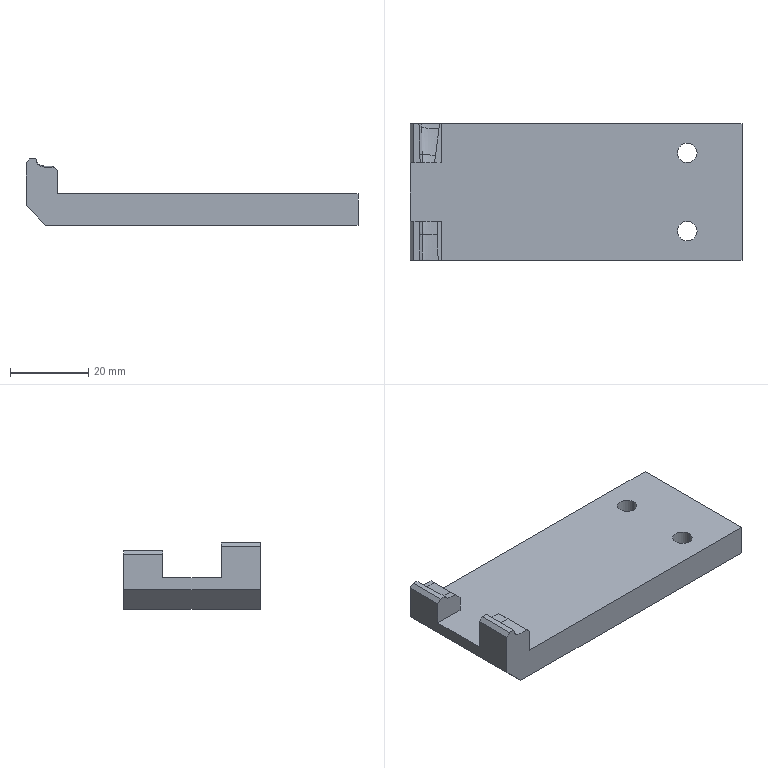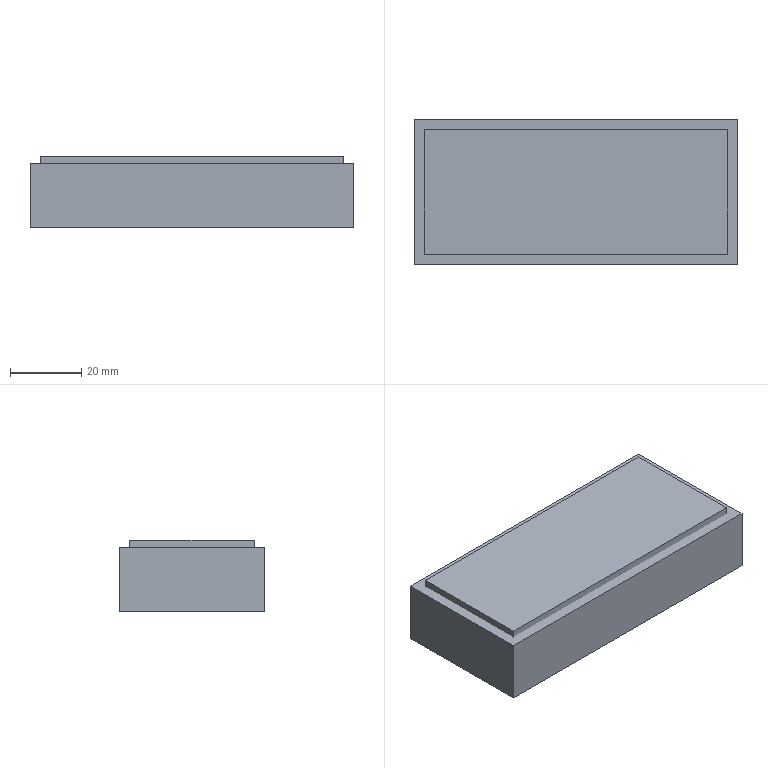CAM job | NX | 3-axis milling, drilling | part box 85 x 35 x 17 mm | stock box 91 x 41 x 20 mm
Tools:
number,name,description,diameter,corner_radius,flute_length,length,flutes
1,D63,Milling Tool-5 Parameters,63.0,0.0,50.0,75.0,2
10,D10,Milling Tool-5 Parameters,10.0,0.0,50.0,75.0,2
11,D10JING,Milling Tool-5 Parameters,10.0,0.0,50.0,75.0,2
7,D6A45,Milling Tool-5 Parameters,6.0,0.0,3.0,3.0,2
14,4.8ZT,Drilling Tool,4.8,0.0,35.0,50.0,2
15,5.0JD,Milling Tool-5 Parameters,5.0,0.0,30.0,30.0,4
5,D3.5R0.5,Milling Tool-5 Parameters,3.5,0.5,50.0,75.0,2
5,D6R0.5,Milling Tool-5 Parameters,6.0,0.5,50.0,75.0,2
Operations:
program,operation,operation_type,tool,method,geometry_group,spindle_rpm,surface_speed,feed_per_tooth,feed_cut,feed_plunge,cut_length_mm,path_length_mm,cut_time_min,machine_time_min
1-90-40-20毛胚,FLOOR_WALL,VolumeBased25DMillingOperation,D63,METHOD,A,6500.0,1286.0,0.0962,1250.0,100.0,166.0,220.0,0.1328,0.1382
1-90-40-20毛胚,ADAPTIVE_MILLING,CavityMilling,D10,METHOD,A,9500.0,298.0,0.1579,3000.0,1000.0,6695.357,7787.36,2.24,2.35
1-90-40-20毛胚,ZLEVEL_PROFILE_COPY_COPY_1_COPY,ZLevelMilling,D10JING,METHOD,A,9500.0,298.0,0.0632,1200.0,100.0,279.437,367.437,0.2329,0.2417
1-90-40-20毛胚,DRILLING_COPY_1,Operation,D6A45,METHOD,A,5000.0,94.0,0.025,250.0,0.0,8.0,117.224,0.032,0.0429
1-90-40-20毛胚,DRILLING_COPY_COPY_1,Operation,4.8ZT,METHOD,A,2000.0,15.0,0.03,120.0,0.0,27.884,156.992,0.2324,0.2453
1-90-40-20毛胚,DRILLING_COPY_COPY_1_COPY,Operation,5.0JD,METHOD,A,1000.0,15.0,0.0125,50.0,0.0,23.0,147.224,0.46,0.4724
1-90-40-20毛胚,FLOOR_WALL_1,VolumeBased25DMillingOperation,D10JING,METHOD,A,9500.0,179.0,0.0658,1250.0,100.0,1023.288,1525.145,0.8186,0.8688
1-90-40-20毛胚,ZLEVEL_PROFILE_COPY_1_COPY_1_COPY_1,ZLevelMilling,D3.5R0.5,METHOD,A,9500.0,119.0,0.1053,2000.0,800.0,1898.852,2098.421,0.9548,0.9748
1-90-40-20毛胚,ZLEVEL_PROFILE_COPY_1_COPY_1_COPY_1_COPY,ZLevelMilling,D3.5R0.5,METHOD,A,9500.0,119.0,0.1053,2000.0,800.0,236.174,298.688,0.1199,0.1261
1-90-40-20毛胚,ZLEVEL_PROFILE_COPY_1_COPY_1_COPY_1_COPY_COPY,ZLevelMilling,D3.5R0.5,METHOD,A,9500.0,119.0,0.1053,2000.0,800.0,235.943,294.457,0.1198,0.1256
1-90-40-20毛胚,ZLEVEL_PROFILE_COPY_1_COPY_1_COPY_1_COPY_COPY_COPY,ZLevelMilling,D3.5R0.5,METHOD,A,9500.0,119.0,0.1053,2000.0,800.0,1436.513,1622.961,0.7236,0.7422
1-90-40-20毛胚,ZLEVEL_PROFILE_1_COPY_1_COPY_COPY,ZLevelMilling,D6A45,METHOD,A,9500.0,179.0,0.0526,1000.0,100.0,234.78,648.324,0.2348,0.2761
2-90-40-20毛胚,FLOOR_WALL_COPY,VolumeBased25DMillingOperation,D63,METHOD,B,6500.0,1286.0,0.0962,1250.0,100.0,480.0,944.001,0.384,0.4304
2-90-40-20毛胚,ZLEVEL_PROFILE_COPY_1_COPY_1_COPY_1_1,ZLevelMilling,D6R0.5,METHOD,B,9500.0,119.0,0.1053,2000.0,800.0,2799.698,2942.243,1.405,1.419
2-90-40-20毛胚,ZLEVEL_PROFILE_1_COPY_1_COPY_COPY_1,ZLevelMilling,D6A45,METHOD,B,9500.0,179.0,0.0526,1000.0,100.0,232.758,506.743,0.2328,0.2602